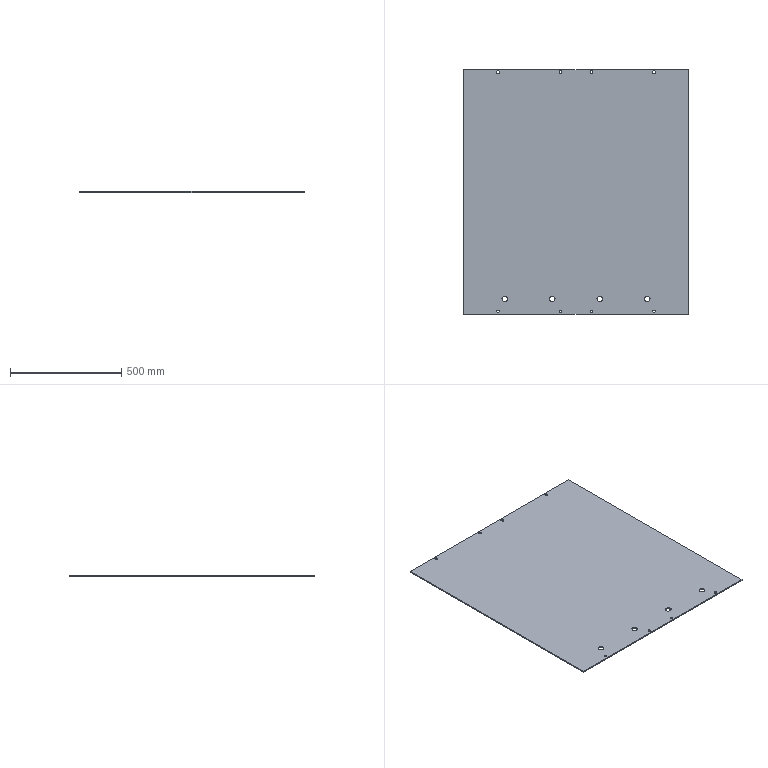Part | STEP file | 750038315 | 1 solid | 38 faces | box 1009 x 1100 x 5 mm | volume 5535001 mm3 | cylinder 24 | plane 14 | commonest cylinder face diameters 11 x16 25 x8
STEP:
#1=CARTESIAN_POINT('',(307.5,70.,0.));
#2=VERTEX_POINT('',#1);
#3=CARTESIAN_POINT('',(332.5,70.,0.));
#4=VERTEX_POINT('',#3);
#5=CARTESIAN_POINT('',(320.,70.,0.));
#6=DIRECTION('',(0.,0.,1.));
#7=DIRECTION('',(1.,0.,0.));
#8=AXIS2_PLACEMENT_3D('',#5,#6,#7);
#9=CIRCLE('',#8,12.5);
#10=EDGE_CURVE('',#2,#4,#9,.T.);
#11=ORIENTED_EDGE('',*,*,#10,.F.);
#12=CARTESIAN_POINT('',(307.5,70.,5.));
#13=VERTEX_POINT('',#12);
#14=CARTESIAN_POINT('',(307.5,70.,-1487.684));
#15=DIRECTION('',(0.,0.,1.));
#16=VECTOR('',#15,1000.);
#17=LINE('',#14,#16);
#18=EDGE_CURVE('',#2,#13,#17,.T.);
#19=ORIENTED_EDGE('',*,*,#18,.T.);
#20=CARTESIAN_POINT('',(332.5,70.,5.));
#21=VERTEX_POINT('',#20);
#22=CARTESIAN_POINT('',(320.,70.,5.));
#23=DIRECTION('',(0.,0.,-1.));
#24=DIRECTION('',(1.,0.,0.));
#25=AXIS2_PLACEMENT_3D('',#22,#23,#24);
#26=CIRCLE('',#25,12.5);
#27=EDGE_CURVE('',#21,#13,#26,.T.);
#28=ORIENTED_EDGE('',*,*,#27,.F.);
#29=CARTESIAN_POINT('',(332.5,70.,-1487.684));
#30=DIRECTION('',(0.,0.,1.));
#31=VECTOR('',#30,1000.);
#32=LINE('',#29,#31);
#33=EDGE_CURVE('',#4,#21,#32,.T.);
#34=ORIENTED_EDGE('',*,*,#33,.F.);
#35=EDGE_LOOP('',(#11,#19,#28,#34));
#36=FACE_OUTER_BOUND('',#35,.T.);
#37=CARTESIAN_POINT('',(320.,70.,-1487.684));
#38=DIRECTION('',(0.,0.,1.));
#39=DIRECTION('',(1.,0.,0.));
#40=AXIS2_PLACEMENT_3D('',#37,#38,#39);
#41=CYLINDRICAL_SURFACE('',#40,12.5);
#42=ADVANCED_FACE('',(#36),#41,.F.);
#43=CARTESIAN_POINT('',(94.167,70.,0.));
#44=VERTEX_POINT('',#43);
#45=CARTESIAN_POINT('',(119.167,70.,0.));
#46=VERTEX_POINT('',#45);
#47=CARTESIAN_POINT('',(106.667,70.,0.));
#48=DIRECTION('',(0.,0.,1.));
#49=DIRECTION('',(1.,0.,0.));
#50=AXIS2_PLACEMENT_3D('',#47,#48,#49);
#51=CIRCLE('',#50,12.5);
#52=EDGE_CURVE('',#44,#46,#51,.T.);
#53=ORIENTED_EDGE('',*,*,#52,.F.);
#54=CARTESIAN_POINT('',(94.167,70.,5.));
#55=VERTEX_POINT('',#54);
#56=CARTESIAN_POINT('',(94.167,70.,-1487.684));
#57=DIRECTION('',(0.,0.,1.));
#58=VECTOR('',#57,1000.);
#59=LINE('',#56,#58);
#60=EDGE_CURVE('',#44,#55,#59,.T.);
#61=ORIENTED_EDGE('',*,*,#60,.T.);
#62=CARTESIAN_POINT('',(119.167,70.,5.));
#63=VERTEX_POINT('',#62);
#64=CARTESIAN_POINT('',(106.667,70.,5.));
#65=DIRECTION('',(0.,0.,-1.));
#66=DIRECTION('',(1.,0.,0.));
#67=AXIS2_PLACEMENT_3D('',#64,#65,#66);
#68=CIRCLE('',#67,12.5);
#69=EDGE_CURVE('',#63,#55,#68,.T.);
#70=ORIENTED_EDGE('',*,*,#69,.F.);
#71=CARTESIAN_POINT('',(119.167,70.,-1487.684));
#72=DIRECTION('',(0.,0.,1.));
#73=VECTOR('',#72,1000.);
#74=LINE('',#71,#73);
#75=EDGE_CURVE('',#46,#63,#74,.T.);
#76=ORIENTED_EDGE('',*,*,#75,.F.);
#77=EDGE_LOOP('',(#53,#61,#70,#76));
#78=FACE_OUTER_BOUND('',#77,.T.);
#79=CARTESIAN_POINT('',(106.667,70.,-1487.684));
#80=DIRECTION('',(0.,0.,1.));
#81=DIRECTION('',(1.,0.,0.));
#82=AXIS2_PLACEMENT_3D('',#79,#80,#81);
#83=CYLINDRICAL_SURFACE('',#82,12.5);
#84=ADVANCED_FACE('',(#78),#83,.F.);
#85=CARTESIAN_POINT('',(-119.167,70.,0.));
#86=VERTEX_POINT('',#85);
#87=CARTESIAN_POINT('',(-94.167,70.,0.));
#88=VERTEX_POINT('',#87);
#89=CARTESIAN_POINT('',(-106.667,70.,0.));
#90=DIRECTION('',(0.,0.,1.));
#91=DIRECTION('',(1.,0.,0.));
#92=AXIS2_PLACEMENT_3D('',#89,#90,#91);
#93=CIRCLE('',#92,12.5);
#94=EDGE_CURVE('',#86,#88,#93,.T.);
#95=ORIENTED_EDGE('',*,*,#94,.F.);
#96=CARTESIAN_POINT('',(-119.167,70.,5.));
#97=VERTEX_POINT('',#96);
#98=CARTESIAN_POINT('',(-119.167,70.,-1487.684));
#99=DIRECTION('',(0.,0.,1.));
#100=VECTOR('',#99,1000.);
#101=LINE('',#98,#100);
#102=EDGE_CURVE('',#86,#97,#101,.T.);
#103=ORIENTED_EDGE('',*,*,#102,.T.);
#104=CARTESIAN_POINT('',(-94.167,70.,5.));
#105=VERTEX_POINT('',#104);
#106=CARTESIAN_POINT('',(-106.667,70.,5.));
#107=DIRECTION('',(0.,0.,-1.));
#108=DIRECTION('',(1.,0.,0.));
#109=AXIS2_PLACEMENT_3D('',#106,#107,#108);
#110=CIRCLE('',#109,12.5);
#111=EDGE_CURVE('',#105,#97,#110,.T.);
#112=ORIENTED_EDGE('',*,*,#111,.F.);
#113=CARTESIAN_POINT('',(-94.167,70.,-1487.684));
#114=DIRECTION('',(0.,0.,1.));
#115=VECTOR('',#114,1000.);
#116=LINE('',#113,#115);
#117=EDGE_CURVE('',#88,#105,#116,.T.);
#118=ORIENTED_EDGE('',*,*,#117,.F.);
#119=EDGE_LOOP('',(#95,#103,#112,#118));
#120=FACE_OUTER_BOUND('',#119,.T.);
#121=CARTESIAN_POINT('',(-106.667,70.,-1487.684));
#122=DIRECTION('',(0.,0.,1.));
#123=DIRECTION('',(1.,0.,0.));
#124=AXIS2_PLACEMENT_3D('',#121,#122,#123);
#125=CYLINDRICAL_SURFACE('',#124,12.5);
#126=ADVANCED_FACE('',(#120),#125,.F.);
#127=CARTESIAN_POINT('',(-332.5,70.,0.));
#128=VERTEX_POINT('',#127);
#129=CARTESIAN_POINT('',(-307.5,70.,0.));
#130=VERTEX_POINT('',#129);
#131=CARTESIAN_POINT('',(-320.,70.,0.));
#132=DIRECTION('',(0.,0.,1.));
#133=DIRECTION('',(1.,0.,0.));
#134=AXIS2_PLACEMENT_3D('',#131,#132,#133);
#135=CIRCLE('',#134,12.5);
#136=EDGE_CURVE('',#128,#130,#135,.T.);
#137=ORIENTED_EDGE('',*,*,#136,.F.);
#138=CARTESIAN_POINT('',(-332.5,70.,5.));
#139=VERTEX_POINT('',#138);
#140=CARTESIAN_POINT('',(-332.5,70.,-1487.684));
#141=DIRECTION('',(0.,0.,1.));
#142=VECTOR('',#141,1000.);
#143=LINE('',#140,#142);
#144=EDGE_CURVE('',#128,#139,#143,.T.);
#145=ORIENTED_EDGE('',*,*,#144,.T.);
#146=CARTESIAN_POINT('',(-307.5,70.,5.));
#147=VERTEX_POINT('',#146);
#148=CARTESIAN_POINT('',(-320.,70.,5.));
#149=DIRECTION('',(0.,0.,-1.));
#150=DIRECTION('',(1.,0.,0.));
#151=AXIS2_PLACEMENT_3D('',#148,#149,#150);
#152=CIRCLE('',#151,12.5);
#153=EDGE_CURVE('',#147,#139,#152,.T.);
#154=ORIENTED_EDGE('',*,*,#153,.F.);
#155=CARTESIAN_POINT('',(-307.5,70.,-1487.684));
#156=DIRECTION('',(0.,0.,1.));
#157=VECTOR('',#156,1000.);
#158=LINE('',#155,#157);
#159=EDGE_CURVE('',#130,#147,#158,.T.);
#160=ORIENTED_EDGE('',*,*,#159,.F.);
#161=EDGE_LOOP('',(#137,#145,#154,#160));
#162=FACE_OUTER_BOUND('',#161,.T.);
#163=CARTESIAN_POINT('',(-320.,70.,-1487.684));
#164=DIRECTION('',(0.,0.,1.));
#165=DIRECTION('',(1.,0.,0.));
#166=AXIS2_PLACEMENT_3D('',#163,#164,#165);
#167=CYLINDRICAL_SURFACE('',#166,12.5);
#168=ADVANCED_FACE('',(#162),#167,.F.);
#169=CARTESIAN_POINT('',(75.5,14.,5.));
#170=VERTEX_POINT('',#169);
#171=CARTESIAN_POINT('',(64.5,14.,5.));
#172=VERTEX_POINT('',#171);
#173=CARTESIAN_POINT('',(70.,14.,5.));
#174=DIRECTION('',(0.,0.,-1.));
#175=DIRECTION('',(-1.,0.,0.));
#176=AXIS2_PLACEMENT_3D('',#173,#174,#175);
#177=CIRCLE('',#176,5.5);
#178=EDGE_CURVE('',#170,#172,#177,.T.);
#179=ORIENTED_EDGE('',*,*,#178,.F.);
#180=CARTESIAN_POINT('',(75.5,14.,0.));
#181=VERTEX_POINT('',#180);
#182=CARTESIAN_POINT('',(75.5,14.,1492.684));
#183=DIRECTION('',(0.,0.,-1.));
#184=VECTOR('',#183,1000.);
#185=LINE('',#182,#184);
#186=EDGE_CURVE('',#170,#181,#185,.T.);
#187=ORIENTED_EDGE('',*,*,#186,.T.);
#188=CARTESIAN_POINT('',(64.5,14.,0.));
#189=VERTEX_POINT('',#188);
#190=CARTESIAN_POINT('',(70.,14.,0.));
#191=DIRECTION('',(0.,0.,1.));
#192=DIRECTION('',(-1.,0.,0.));
#193=AXIS2_PLACEMENT_3D('',#190,#191,#192);
#194=CIRCLE('',#193,5.5);
#195=EDGE_CURVE('',#189,#181,#194,.T.);
#196=ORIENTED_EDGE('',*,*,#195,.F.);
#197=CARTESIAN_POINT('',(64.5,14.,1492.684));
#198=DIRECTION('',(0.,0.,-1.));
#199=VECTOR('',#198,1000.);
#200=LINE('',#197,#199);
#201=EDGE_CURVE('',#172,#189,#200,.T.);
#202=ORIENTED_EDGE('',*,*,#201,.F.);
#203=EDGE_LOOP('',(#179,#187,#196,#202));
#204=FACE_OUTER_BOUND('',#203,.T.);
#205=CARTESIAN_POINT('',(70.,14.,1492.684));
#206=DIRECTION('',(0.,0.,-1.));
#207=DIRECTION('',(-1.,0.,0.));
#208=AXIS2_PLACEMENT_3D('',#205,#206,#207);
#209=CYLINDRICAL_SURFACE('',#208,5.5);
#210=ADVANCED_FACE('',(#204),#209,.F.);
#211=CARTESIAN_POINT('',(-64.5,14.,5.));
#212=VERTEX_POINT('',#211);
#213=CARTESIAN_POINT('',(-75.5,14.,5.));
#214=VERTEX_POINT('',#213);
#215=CARTESIAN_POINT('',(-70.,14.,5.));
#216=DIRECTION('',(0.,0.,-1.));
#217=DIRECTION('',(-1.,0.,0.));
#218=AXIS2_PLACEMENT_3D('',#215,#216,#217);
#219=CIRCLE('',#218,5.5);
#220=EDGE_CURVE('',#212,#214,#219,.T.);
#221=ORIENTED_EDGE('',*,*,#220,.F.);
#222=CARTESIAN_POINT('',(-64.5,14.,0.));
#223=VERTEX_POINT('',#222);
#224=CARTESIAN_POINT('',(-64.5,14.,1492.684));
#225=DIRECTION('',(0.,0.,-1.));
#226=VECTOR('',#225,1000.);
#227=LINE('',#224,#226);
#228=EDGE_CURVE('',#212,#223,#227,.T.);
#229=ORIENTED_EDGE('',*,*,#228,.T.);
#230=CARTESIAN_POINT('',(-75.5,14.,0.));
#231=VERTEX_POINT('',#230);
#232=CARTESIAN_POINT('',(-70.,14.,0.));
#233=DIRECTION('',(0.,0.,1.));
#234=DIRECTION('',(-1.,0.,0.));
#235=AXIS2_PLACEMENT_3D('',#232,#233,#234);
#236=CIRCLE('',#235,5.5);
#237=EDGE_CURVE('',#231,#223,#236,.T.);
#238=ORIENTED_EDGE('',*,*,#237,.F.);
#239=CARTESIAN_POINT('',(-75.5,14.,1492.684));
#240=DIRECTION('',(0.,0.,-1.));
#241=VECTOR('',#240,1000.);
#242=LINE('',#239,#241);
#243=EDGE_CURVE('',#214,#231,#242,.T.);
#244=ORIENTED_EDGE('',*,*,#243,.F.);
#245=EDGE_LOOP('',(#221,#229,#238,#244));
#246=FACE_OUTER_BOUND('',#245,.T.);
#247=CARTESIAN_POINT('',(-70.,14.,1492.684));
#248=DIRECTION('',(0.,0.,-1.));
#249=DIRECTION('',(-1.,0.,0.));
#250=AXIS2_PLACEMENT_3D('',#247,#248,#249);
#251=CYLINDRICAL_SURFACE('',#250,5.5);
#252=ADVANCED_FACE('',(#246),#251,.F.);
#253=CARTESIAN_POINT('',(-344.5,14.,5.));
#254=VERTEX_POINT('',#253);
#255=CARTESIAN_POINT('',(-355.5,14.,5.));
#256=VERTEX_POINT('',#255);
#257=CARTESIAN_POINT('',(-350.,14.,5.));
#258=DIRECTION('',(0.,0.,-1.));
#259=DIRECTION('',(-1.,0.,0.));
#260=AXIS2_PLACEMENT_3D('',#257,#258,#259);
#261=CIRCLE('',#260,5.5);
#262=EDGE_CURVE('',#254,#256,#261,.T.);
#263=ORIENTED_EDGE('',*,*,#262,.F.);
#264=CARTESIAN_POINT('',(-344.5,14.,0.));
#265=VERTEX_POINT('',#264);
#266=CARTESIAN_POINT('',(-344.5,14.,1492.684));
#267=DIRECTION('',(0.,0.,-1.));
#268=VECTOR('',#267,1000.);
#269=LINE('',#266,#268);
#270=EDGE_CURVE('',#254,#265,#269,.T.);
#271=ORIENTED_EDGE('',*,*,#270,.T.);
#272=CARTESIAN_POINT('',(-355.5,14.,0.));
#273=VERTEX_POINT('',#272);
#274=CARTESIAN_POINT('',(-350.,14.,0.));
#275=DIRECTION('',(0.,0.,1.));
#276=DIRECTION('',(-1.,0.,0.));
#277=AXIS2_PLACEMENT_3D('',#274,#275,#276);
#278=CIRCLE('',#277,5.5);
#279=EDGE_CURVE('',#273,#265,#278,.T.);
#280=ORIENTED_EDGE('',*,*,#279,.F.);
#281=CARTESIAN_POINT('',(-355.5,14.,1492.684));
#282=DIRECTION('',(0.,0.,-1.));
#283=VECTOR('',#282,1000.);
#284=LINE('',#281,#283);
#285=EDGE_CURVE('',#256,#273,#284,.T.);
#286=ORIENTED_EDGE('',*,*,#285,.F.);
#287=EDGE_LOOP('',(#263,#271,#280,#286));
#288=FACE_OUTER_BOUND('',#287,.T.);
#289=CARTESIAN_POINT('',(-350.,14.,1492.684));
#290=DIRECTION('',(0.,0.,-1.));
#291=DIRECTION('',(-1.,0.,0.));
#292=AXIS2_PLACEMENT_3D('',#289,#290,#291);
#293=CYLINDRICAL_SURFACE('',#292,5.5);
#294=ADVANCED_FACE('',(#288),#293,.F.);
#295=CARTESIAN_POINT('',(355.5,14.,5.));
#296=VERTEX_POINT('',#295);
#297=CARTESIAN_POINT('',(344.5,14.,5.));
#298=VERTEX_POINT('',#297);
#299=CARTESIAN_POINT('',(350.,14.,5.));
#300=DIRECTION('',(0.,0.,-1.));
#301=DIRECTION('',(-1.,0.,0.));
#302=AXIS2_PLACEMENT_3D('',#299,#300,#301);
#303=CIRCLE('',#302,5.5);
#304=EDGE_CURVE('',#296,#298,#303,.T.);
#305=ORIENTED_EDGE('',*,*,#304,.F.);
#306=CARTESIAN_POINT('',(355.5,14.,0.));
#307=VERTEX_POINT('',#306);
#308=CARTESIAN_POINT('',(355.5,14.,1492.684));
#309=DIRECTION('',(0.,0.,-1.));
#310=VECTOR('',#309,1000.);
#311=LINE('',#308,#310);
#312=EDGE_CURVE('',#296,#307,#311,.T.);
#313=ORIENTED_EDGE('',*,*,#312,.T.);
#314=CARTESIAN_POINT('',(344.5,14.,0.));
#315=VERTEX_POINT('',#314);
#316=CARTESIAN_POINT('',(350.,14.,0.));
#317=DIRECTION('',(0.,0.,1.));
#318=DIRECTION('',(-1.,0.,0.));
#319=AXIS2_PLACEMENT_3D('',#316,#317,#318);
#320=CIRCLE('',#319,5.5);
#321=EDGE_CURVE('',#315,#307,#320,.T.);
#322=ORIENTED_EDGE('',*,*,#321,.F.);
#323=CARTESIAN_POINT('',(344.5,14.,1492.684));
#324=DIRECTION('',(0.,0.,-1.));
#325=VECTOR('',#324,1000.);
#326=LINE('',#323,#325);
#327=EDGE_CURVE('',#298,#315,#326,.T.);
#328=ORIENTED_EDGE('',*,*,#327,.F.);
#329=EDGE_LOOP('',(#305,#313,#322,#328));
#330=FACE_OUTER_BOUND('',#329,.T.);
#331=CARTESIAN_POINT('',(350.,14.,1492.684));
#332=DIRECTION('',(0.,0.,-1.));
#333=DIRECTION('',(-1.,0.,0.));
#334=AXIS2_PLACEMENT_3D('',#331,#332,#333);
#335=CYLINDRICAL_SURFACE('',#334,5.5);
#336=ADVANCED_FACE('',(#330),#335,.F.);
#337=CARTESIAN_POINT('',(-355.5,1090.,0.));
#338=VERTEX_POINT('',#337);
#339=CARTESIAN_POINT('',(-355.5,1086.,0.));
#340=VERTEX_POINT('',#339);
#341=CARTESIAN_POINT('',(-355.5,0.,0.));
#342=DIRECTION('',(0.,-1.,0.));
#343=VECTOR('',#342,1000.);
#344=LINE('',#341,#343);
#345=EDGE_CURVE('',#338,#340,#344,.T.);
#346=ORIENTED_EDGE('',*,*,#345,.T.);
#347=CARTESIAN_POINT('',(-344.5,1086.,0.));
#348=VERTEX_POINT('',#347);
#349=CARTESIAN_POINT('',(-350.,1086.,0.));
#350=DIRECTION('',(0.,0.,1.));
#351=DIRECTION('',(-1.,0.,0.));
#352=AXIS2_PLACEMENT_3D('',#349,#350,#351);
#353=CIRCLE('',#352,5.5);
#354=EDGE_CURVE('',#340,#348,#353,.T.);
#355=ORIENTED_EDGE('',*,*,#354,.T.);
#356=CARTESIAN_POINT('',(-344.5,1090.,0.));
#357=VERTEX_POINT('',#356);
#358=CARTESIAN_POINT('',(-344.5,0.,0.));
#359=DIRECTION('',(0.,1.,0.));
#360=VECTOR('',#359,1000.);
#361=LINE('',#358,#360);
#362=EDGE_CURVE('',#348,#357,#361,.T.);
#363=ORIENTED_EDGE('',*,*,#362,.T.);
#364=CARTESIAN_POINT('',(-350.,1090.,0.));
#365=DIRECTION('',(0.,0.,1.));
#366=DIRECTION('',(-1.,0.,0.));
#367=AXIS2_PLACEMENT_3D('',#364,#365,#366);
#368=CIRCLE('',#367,5.5);
#369=EDGE_CURVE('',#357,#338,#368,.T.);
#370=ORIENTED_EDGE('',*,*,#369,.T.);
#371=EDGE_LOOP('',(#346,#355,#363,#370));
#372=FACE_BOUND('',#371,.T.);
#373=CARTESIAN_POINT('',(-75.5,1090.,0.));
#374=VERTEX_POINT('',#373);
#375=CARTESIAN_POINT('',(-75.5,1086.,0.));
#376=VERTEX_POINT('',#375);
#377=CARTESIAN_POINT('',(-75.5,0.,0.));
#378=DIRECTION('',(0.,-1.,0.));
#379=VECTOR('',#378,1000.);
#380=LINE('',#377,#379);
#381=EDGE_CURVE('',#374,#376,#380,.T.);
#382=ORIENTED_EDGE('',*,*,#381,.T.);
#383=CARTESIAN_POINT('',(-64.5,1086.,0.));
#384=VERTEX_POINT('',#383);
#385=CARTESIAN_POINT('',(-70.,1086.,0.));
#386=DIRECTION('',(0.,0.,1.));
#387=DIRECTION('',(-1.,0.,0.));
#388=AXIS2_PLACEMENT_3D('',#385,#386,#387);
#389=CIRCLE('',#388,5.5);
#390=EDGE_CURVE('',#376,#384,#389,.T.);
#391=ORIENTED_EDGE('',*,*,#390,.T.);
#392=CARTESIAN_POINT('',(-64.5,1090.,0.));
#393=VERTEX_POINT('',#392);
#394=CARTESIAN_POINT('',(-64.5,0.,0.));
#395=DIRECTION('',(0.,1.,0.));
#396=VECTOR('',#395,1000.);
#397=LINE('',#394,#396);
#398=EDGE_CURVE('',#384,#393,#397,.T.);
#399=ORIENTED_EDGE('',*,*,#398,.T.);
#400=CARTESIAN_POINT('',(-70.,1090.,0.));
#401=DIRECTION('',(0.,0.,1.));
#402=DIRECTION('',(-1.,0.,0.));
#403=AXIS2_PLACEMENT_3D('',#400,#401,#402);
#404=CIRCLE('',#403,5.5);
#405=EDGE_CURVE('',#393,#374,#404,.T.);
#406=ORIENTED_EDGE('',*,*,#405,.T.);
#407=EDGE_LOOP('',(#382,#391,#399,#406));
#408=FACE_BOUND('',#407,.T.);
#409=CARTESIAN_POINT('',(64.5,1090.,0.));
#410=VERTEX_POINT('',#409);
#411=CARTESIAN_POINT('',(64.5,1086.,0.));
#412=VERTEX_POINT('',#411);
#413=CARTESIAN_POINT('',(64.5,0.,0.));
#414=DIRECTION('',(0.,-1.,0.));
#415=VECTOR('',#414,1000.);
#416=LINE('',#413,#415);
#417=EDGE_CURVE('',#410,#412,#416,.T.);
#418=ORIENTED_EDGE('',*,*,#417,.T.);
#419=CARTESIAN_POINT('',(75.5,1086.,0.));
#420=VERTEX_POINT('',#419);
#421=CARTESIAN_POINT('',(70.,1086.,0.));
#422=DIRECTION('',(0.,0.,1.));
#423=DIRECTION('',(-1.,0.,0.));
#424=AXIS2_PLACEMENT_3D('',#421,#422,#423);
#425=CIRCLE('',#424,5.5);
#426=EDGE_CURVE('',#412,#420,#425,.T.);
#427=ORIENTED_EDGE('',*,*,#426,.T.);
#428=CARTESIAN_POINT('',(75.5,1090.,0.));
#429=VERTEX_POINT('',#428);
#430=CARTESIAN_POINT('',(75.5,0.,0.));
#431=DIRECTION('',(0.,1.,0.));
#432=VECTOR('',#431,1000.);
#433=LINE('',#430,#432);
#434=EDGE_CURVE('',#420,#429,#433,.T.);
#435=ORIENTED_EDGE('',*,*,#434,.T.);
#436=CARTESIAN_POINT('',(70.,1090.,0.));
#437=DIRECTION('',(0.,0.,1.));
#438=DIRECTION('',(-1.,0.,0.));
#439=AXIS2_PLACEMENT_3D('',#436,#437,#438);
#440=CIRCLE('',#439,5.5);
#441=EDGE_CURVE('',#429,#410,#440,.T.);
#442=ORIENTED_EDGE('',*,*,#441,.T.);
#443=EDGE_LOOP('',(#418,#427,#435,#442));
#444=FACE_BOUND('',#443,.T.);
#445=CARTESIAN_POINT('',(344.5,1090.,0.));
#446=VERTEX_POINT('',#445);
#447=CARTESIAN_POINT('',(344.5,1086.,0.));
#448=VERTEX_POINT('',#447);
#449=CARTESIAN_POINT('',(344.5,0.,0.));
#450=DIRECTION('',(0.,-1.,0.));
#451=VECTOR('',#450,1000.);
#452=LINE('',#449,#451);
#453=EDGE_CURVE('',#446,#448,#452,.T.);
#454=ORIENTED_EDGE('',*,*,#453,.T.);
#455=CARTESIAN_POINT('',(355.5,1086.,0.));
#456=VERTEX_POINT('',#455);
#457=CARTESIAN_POINT('',(350.,1086.,0.));
#458=DIRECTION('',(0.,0.,1.));
#459=DIRECTION('',(-1.,0.,0.));
#460=AXIS2_PLACEMENT_3D('',#457,#458,#459);
#461=CIRCLE('',#460,5.5);
#462=EDGE_CURVE('',#448,#456,#461,.T.);
#463=ORIENTED_EDGE('',*,*,#462,.T.);
#464=CARTESIAN_POINT('',(355.5,1090.,0.));
#465=VERTEX_POINT('',#464);
#466=CARTESIAN_POINT('',(355.5,0.,0.));
#467=DIRECTION('',(0.,1.,0.));
#468=VECTOR('',#467,1000.);
#469=LINE('',#466,#468);
#470=EDGE_CURVE('',#456,#465,#469,.T.);
#471=ORIENTED_EDGE('',*,*,#470,.T.);
#472=CARTESIAN_POINT('',(350.,1090.,0.));
#473=DIRECTION('',(0.,0.,1.));
#474=DIRECTION('',(-1.,0.,0.));
#475=AXIS2_PLACEMENT_3D('',#472,#473,#474);
#476=CIRCLE('',#475,5.5);
#477=EDGE_CURVE('',#465,#446,#476,.T.);
#478=ORIENTED_EDGE('',*,*,#477,.T.);
#479=EDGE_LOOP('',(#454,#463,#471,#478));
#480=FACE_BOUND('',#479,.T.);
#481=CARTESIAN_POINT('',(-504.5,1100.,0.));
#482=VERTEX_POINT('',#481);
#483=CARTESIAN_POINT('',(504.5,1100.,0.));
#484=VERTEX_POINT('',#483);
#485=CARTESIAN_POINT('',(0.,1100.,0.));
#486=DIRECTION('',(1.,0.,0.));
#487=VECTOR('',#486,1000.);
#488=LINE('',#485,#487);
#489=EDGE_CURVE('',#482,#484,#488,.T.);
#490=ORIENTED_EDGE('',*,*,#489,.T.);
#491=CARTESIAN_POINT('',(504.5,0.,0.));
#492=VERTEX_POINT('',#491);
#493=CARTESIAN_POINT('',(504.5,0.,0.));
#494=DIRECTION('',(0.,-1.,0.));
#495=VECTOR('',#494,1000.);
#496=LINE('',#493,#495);
#497=EDGE_CURVE('',#484,#492,#496,.T.);
#498=ORIENTED_EDGE('',*,*,#497,.T.);
#499=CARTESIAN_POINT('',(-504.5,0.,0.));
#500=VERTEX_POINT('',#499);
#501=CARTESIAN_POINT('',(0.,0.,0.));
#502=DIRECTION('',(-1.,0.,0.));
#503=VECTOR('',#502,1000.);
#504=LINE('',#501,#503);
#505=EDGE_CURVE('',#492,#500,#504,.T.);
#506=ORIENTED_EDGE('',*,*,#505,.T.);
#507=CARTESIAN_POINT('',(-504.5,0.,0.));
#508=DIRECTION('',(0.,1.,0.));
#509=VECTOR('',#508,1000.);
#510=LINE('',#507,#509);
#511=EDGE_CURVE('',#500,#482,#510,.T.);
#512=ORIENTED_EDGE('',*,*,#511,.T.);
#513=EDGE_LOOP('',(#490,#498,#506,#512));
#514=FACE_OUTER_BOUND('',#513,.T.);
#515=CARTESIAN_POINT('',(320.,70.,0.));
#516=DIRECTION('',(0.,0.,1.));
#517=DIRECTION('',(1.,0.,0.));
#518=AXIS2_PLACEMENT_3D('',#515,#516,#517);
#519=CIRCLE('',#518,12.5);
#520=EDGE_CURVE('',#4,#2,#519,.T.);
#521=ORIENTED_EDGE('',*,*,#520,.T.);
#522=ORIENTED_EDGE('',*,*,#10,.T.);
#523=EDGE_LOOP('',(#521,#522));
#524=FACE_BOUND('',#523,.T.);
#525=CARTESIAN_POINT('',(106.667,70.,0.));
#526=DIRECTION('',(0.,0.,1.));
#527=DIRECTION('',(1.,0.,0.));
#528=AXIS2_PLACEMENT_3D('',#525,#526,#527);
#529=CIRCLE('',#528,12.5);
#530=EDGE_CURVE('',#46,#44,#529,.T.);
#531=ORIENTED_EDGE('',*,*,#530,.T.);
#532=ORIENTED_EDGE('',*,*,#52,.T.);
#533=EDGE_LOOP('',(#531,#532));
#534=FACE_BOUND('',#533,.T.);
#535=CARTESIAN_POINT('',(-106.667,70.,0.));
#536=DIRECTION('',(0.,0.,1.));
#537=DIRECTION('',(1.,0.,0.));
#538=AXIS2_PLACEMENT_3D('',#535,#536,#537);
#539=CIRCLE('',#538,12.5);
#540=EDGE_CURVE('',#88,#86,#539,.T.);
#541=ORIENTED_EDGE('',*,*,#540,.T.);
#542=ORIENTED_EDGE('',*,*,#94,.T.);
#543=EDGE_LOOP('',(#541,#542));
#544=FACE_BOUND('',#543,.T.);
#545=CARTESIAN_POINT('',(-320.,70.,0.));
#546=DIRECTION('',(0.,0.,1.));
#547=DIRECTION('',(1.,0.,0.));
#548=AXIS2_PLACEMENT_3D('',#545,#546,#547);
#549=CIRCLE('',#548,12.5);
#550=EDGE_CURVE('',#130,#128,#549,.T.);
#551=ORIENTED_EDGE('',*,*,#550,.T.);
#552=ORIENTED_EDGE('',*,*,#136,.T.);
#553=EDGE_LOOP('',(#551,#552));
#554=FACE_BOUND('',#553,.T.);
#555=ORIENTED_EDGE('',*,*,#195,.T.);
#556=CARTESIAN_POINT('',(70.,14.,0.));
#557=DIRECTION('',(0.,0.,1.));
#558=DIRECTION('',(-1.,0.,0.));
#559=AXIS2_PLACEMENT_3D('',#556,#557,#558);
#560=CIRCLE('',#559,5.5);
#561=EDGE_CURVE('',#181,#189,#560,.T.);
#562=ORIENTED_EDGE('',*,*,#561,.T.);
#563=EDGE_LOOP('',(#555,#562));
#564=FACE_BOUND('',#563,.T.);
#565=ORIENTED_EDGE('',*,*,#237,.T.);
#566=CARTESIAN_POINT('',(-70.,14.,0.));
#567=DIRECTION('',(0.,0.,1.));
#568=DIRECTION('',(-1.,0.,0.));
#569=AXIS2_PLACEMENT_3D('',#566,#567,#568);
#570=CIRCLE('',#569,5.5);
#571=EDGE_CURVE('',#223,#231,#570,.T.);
#572=ORIENTED_EDGE('',*,*,#571,.T.);
#573=EDGE_LOOP('',(#565,#572));
#574=FACE_BOUND('',#573,.T.);
#575=ORIENTED_EDGE('',*,*,#279,.T.);
#576=CARTESIAN_POINT('',(-350.,14.,0.));
#577=DIRECTION('',(0.,0.,1.));
#578=DIRECTION('',(-1.,0.,0.));
#579=AXIS2_PLACEMENT_3D('',#576,#577,#578);
#580=CIRCLE('',#579,5.5);
#581=EDGE_CURVE('',#265,#273,#580,.T.);
#582=ORIENTED_EDGE('',*,*,#581,.T.);
#583=EDGE_LOOP('',(#575,#582));
#584=FACE_BOUND('',#583,.T.);
#585=ORIENTED_EDGE('',*,*,#321,.T.);
#586=CARTESIAN_POINT('',(350.,14.,0.));
#587=DIRECTION('',(0.,0.,1.));
#588=DIRECTION('',(-1.,0.,0.));
#589=AXIS2_PLACEMENT_3D('',#586,#587,#588);
#590=CIRCLE('',#589,5.5);
#591=EDGE_CURVE('',#307,#315,#590,.T.);
#592=ORIENTED_EDGE('',*,*,#591,.T.);
#593=EDGE_LOOP('',(#585,#592));
#594=FACE_BOUND('',#593,.T.);
#595=CARTESIAN_POINT('',(0.,0.,0.));
#596=DIRECTION('',(0.,0.,-1.));
#597=DIRECTION('',(-1.,0.,0.));
#598=AXIS2_PLACEMENT_3D('',#595,#596,#597);
#599=PLANE('',#598);
#600=ADVANCED_FACE('',(#372,#408,#444,#480,#514,#524,#534,#544,#554,#564,#574,#584,#594),#599,.T.);
#601=CARTESIAN_POINT('',(-344.5,1086.,5.));
#602=VERTEX_POINT('',#601);
#603=CARTESIAN_POINT('',(-344.5,1086.,1492.684));
#604=DIRECTION('',(0.,0.,1.));
#605=VECTOR('',#604,1000.);
#606=LINE('',#603,#605);
#607=EDGE_CURVE('',#348,#602,#606,.T.);
#608=ORIENTED_EDGE('',*,*,#607,.F.);
#609=ORIENTED_EDGE('',*,*,#354,.F.);
#610=CARTESIAN_POINT('',(-355.5,1086.,5.));
#611=VERTEX_POINT('',#610);
#612=CARTESIAN_POINT('',(-355.5,1086.,1492.684));
#613=DIRECTION('',(0.,0.,-1.));
#614=VECTOR('',#613,1000.);
#615=LINE('',#612,#614);
#616=EDGE_CURVE('',#611,#340,#615,.T.);
#617=ORIENTED_EDGE('',*,*,#616,.F.);
#618=CARTESIAN_POINT('',(-350.,1086.,5.));
#619=DIRECTION('',(0.,0.,-1.));
#620=DIRECTION('',(-1.,0.,0.));
#621=AXIS2_PLACEMENT_3D('',#618,#619,#620);
#622=CIRCLE('',#621,5.5);
#623=EDGE_CURVE('',#602,#611,#622,.T.);
#624=ORIENTED_EDGE('',*,*,#623,.F.);
#625=EDGE_LOOP('',(#608,#609,#617,#624));
#626=FACE_OUTER_BOUND('',#625,.T.);
#627=CARTESIAN_POINT('',(-350.,1086.,1492.684));
#628=DIRECTION('',(0.,0.,-1.));
#629=DIRECTION('',(-1.,0.,0.));
#630=AXIS2_PLACEMENT_3D('',#627,#628,#629);
#631=CYLINDRICAL_SURFACE('',#630,5.5);
#632=ADVANCED_FACE('',(#626),#631,.F.);
#633=ORIENTED_EDGE('',*,*,#345,.F.);
#634=CARTESIAN_POINT('',(-355.5,1090.,5.));
#635=VERTEX_POINT('',#634);
#636=CARTESIAN_POINT('',(-355.5,1090.,1492.684));
#637=DIRECTION('',(0.,0.,1.));
#638=VECTOR('',#637,1000.);
#639=LINE('',#636,#638);
#640=EDGE_CURVE('',#338,#635,#639,.T.);
#641=ORIENTED_EDGE('',*,*,#640,.T.);
#642=CARTESIAN_POINT('',(-355.5,1090.,5.));
#643=DIRECTION('',(0.,-1.,0.));
#644=VECTOR('',#643,1000.);
#645=LINE('',#642,#644);
#646=EDGE_CURVE('',#635,#611,#645,.T.);
#647=ORIENTED_EDGE('',*,*,#646,.T.);
#648=ORIENTED_EDGE('',*,*,#616,.T.);
#649=EDGE_LOOP('',(#633,#641,#647,#648));
#650=FACE_OUTER_BOUND('',#649,.T.);
#651=CARTESIAN_POINT('',(-355.5,1090.,1492.684));
#652=DIRECTION('',(1.,0.,0.));
#653=DIRECTION('',(0.,0.,-1.));
#654=AXIS2_PLACEMENT_3D('',#651,#652,#653);
#655=PLANE('',#654);
#656=ADVANCED_FACE('',(#650),#655,.T.);
#657=ORIENTED_EDGE('',*,*,#640,.F.);
#658=ORIENTED_EDGE('',*,*,#369,.F.);
#659=CARTESIAN_POINT('',(-344.5,1090.,5.));
#660=VERTEX_POINT('',#659);
#661=CARTESIAN_POINT('',(-344.5,1090.,1492.684));
#662=DIRECTION('',(0.,0.,-1.));
#663=VECTOR('',#662,1000.);
#664=LINE('',#661,#663);
#665=EDGE_CURVE('',#660,#357,#664,.T.);
#666=ORIENTED_EDGE('',*,*,#665,.F.);
#667=CARTESIAN_POINT('',(-350.,1090.,5.));
#668=DIRECTION('',(0.,0.,-1.));
#669=DIRECTION('',(-1.,0.,0.));
#670=AXIS2_PLACEMENT_3D('',#667,#668,#669);
#671=CIRCLE('',#670,5.5);
#672=EDGE_CURVE('',#635,#660,#671,.T.);
#673=ORIENTED_EDGE('',*,*,#672,.F.);
#674=EDGE_LOOP('',(#657,#658,#666,#673));
#675=FACE_OUTER_BOUND('',#674,.T.);
#676=CARTESIAN_POINT('',(-350.,1090.,1492.684));
#677=DIRECTION('',(0.,0.,-1.));
#678=DIRECTION('',(-1.,0.,0.));
#679=AXIS2_PLACEMENT_3D('',#676,#677,#678);
#680=CYLINDRICAL_SURFACE('',#679,5.5);
#681=ADVANCED_FACE('',(#675),#680,.F.);
#682=ORIENTED_EDGE('',*,*,#362,.F.);
#683=ORIENTED_EDGE('',*,*,#607,.T.);
#684=CARTESIAN_POINT('',(-344.5,1086.,5.));
#685=DIRECTION('',(0.,1.,0.));
#686=VECTOR('',#685,1000.);
#687=LINE('',#684,#686);
#688=EDGE_CURVE('',#602,#660,#687,.T.);
#689=ORIENTED_EDGE('',*,*,#688,.T.);
#690=ORIENTED_EDGE('',*,*,#665,.T.);
#691=EDGE_LOOP('',(#682,#683,#689,#690));
#692=FACE_OUTER_BOUND('',#691,.T.);
#693=CARTESIAN_POINT('',(-344.5,1086.,1492.684));
#694=DIRECTION('',(-1.,0.,0.));
#695=DIRECTION('',(0.,0.,1.));
#696=AXIS2_PLACEMENT_3D('',#693,#694,#695);
#697=PLANE('',#696);
#698=ADVANCED_FACE('',(#692),#697,.T.);
#699=CARTESIAN_POINT('',(-64.5,1086.,5.));
#700=VERTEX_POINT('',#699);
#701=CARTESIAN_POINT('',(-64.5,1086.,1492.684));
#702=DIRECTION('',(0.,0.,1.));
#703=VECTOR('',#702,1000.);
#704=LINE('',#701,#703);
#705=EDGE_CURVE('',#384,#700,#704,.T.);
#706=ORIENTED_EDGE('',*,*,#705,.F.);
#707=ORIENTED_EDGE('',*,*,#390,.F.);
#708=CARTESIAN_POINT('',(-75.5,1086.,5.));
#709=VERTEX_POINT('',#708);
#710=CARTESIAN_POINT('',(-75.5,1086.,1492.684));
#711=DIRECTION('',(0.,0.,-1.));
#712=VECTOR('',#711,1000.);
#713=LINE('',#710,#712);
#714=EDGE_CURVE('',#709,#376,#713,.T.);
#715=ORIENTED_EDGE('',*,*,#714,.F.);
#716=CARTESIAN_POINT('',(-70.,1086.,5.));
#717=DIRECTION('',(0.,0.,-1.));
#718=DIRECTION('',(-1.,0.,0.));
#719=AXIS2_PLACEMENT_3D('',#716,#717,#718);
#720=CIRCLE('',#719,5.5);
#721=EDGE_CURVE('',#700,#709,#720,.T.);
#722=ORIENTED_EDGE('',*,*,#721,.F.);
#723=EDGE_LOOP('',(#706,#707,#715,#722));
#724=FACE_OUTER_BOUND('',#723,.T.);
#725=CARTESIAN_POINT('',(-70.,1086.,1492.684));
#726=DIRECTION('',(0.,0.,-1.));
#727=DIRECTION('',(-1.,0.,0.));
#728=AXIS2_PLACEMENT_3D('',#725,#726,#727);
#729=CYLINDRICAL_SURFACE('',#728,5.5);
#730=ADVANCED_FACE('',(#724),#729,.F.);
#731=ORIENTED_EDGE('',*,*,#381,.F.);
#732=CARTESIAN_POINT('',(-75.5,1090.,5.));
#733=VERTEX_POINT('',#732);
#734=CARTESIAN_POINT('',(-75.5,1090.,1492.684));
#735=DIRECTION('',(0.,0.,1.));
#736=VECTOR('',#735,1000.);
#737=LINE('',#734,#736);
#738=EDGE_CURVE('',#374,#733,#737,.T.);
#739=ORIENTED_EDGE('',*,*,#738,.T.);
#740=CARTESIAN_POINT('',(-75.5,1090.,5.));
#741=DIRECTION('',(0.,-1.,0.));
#742=VECTOR('',#741,1000.);
#743=LINE('',#740,#742);
#744=EDGE_CURVE('',#733,#709,#743,.T.);
#745=ORIENTED_EDGE('',*,*,#744,.T.);
#746=ORIENTED_EDGE('',*,*,#714,.T.);
#747=EDGE_LOOP('',(#731,#739,#745,#746));
#748=FACE_OUTER_BOUND('',#747,.T.);
#749=CARTESIAN_POINT('',(-75.5,1090.,1492.684));
#750=DIRECTION('',(1.,0.,0.));
#751=DIRECTION('',(0.,0.,-1.));
#752=AXIS2_PLACEMENT_3D('',#749,#750,#751);
#753=PLANE('',#752);
#754=ADVANCED_FACE('',(#748),#753,.T.);
#755=ORIENTED_EDGE('',*,*,#738,.F.);
#756=ORIENTED_EDGE('',*,*,#405,.F.);
#757=CARTESIAN_POINT('',(-64.5,1090.,5.));
#758=VERTEX_POINT('',#757);
#759=CARTESIAN_POINT('',(-64.5,1090.,1492.684));
#760=DIRECTION('',(0.,0.,-1.));
#761=VECTOR('',#760,1000.);
#762=LINE('',#759,#761);
#763=EDGE_CURVE('',#758,#393,#762,.T.);
#764=ORIENTED_EDGE('',*,*,#763,.F.);
#765=CARTESIAN_POINT('',(-70.,1090.,5.));
#766=DIRECTION('',(0.,0.,-1.));
#767=DIRECTION('',(-1.,0.,0.));
#768=AXIS2_PLACEMENT_3D('',#765,#766,#767);
#769=CIRCLE('',#768,5.5);
#770=EDGE_CURVE('',#733,#758,#769,.T.);
#771=ORIENTED_EDGE('',*,*,#770,.F.);
#772=EDGE_LOOP('',(#755,#756,#764,#771));
#773=FACE_OUTER_BOUND('',#772,.T.);
#774=CARTESIAN_POINT('',(-70.,1090.,1492.684));
#775=DIRECTION('',(0.,0.,-1.));
#776=DIRECTION('',(-1.,0.,0.));
#777=AXIS2_PLACEMENT_3D('',#774,#775,#776);
#778=CYLINDRICAL_SURFACE('',#777,5.5);
#779=ADVANCED_FACE('',(#773),#778,.F.);
#780=ORIENTED_EDGE('',*,*,#398,.F.);
#781=ORIENTED_EDGE('',*,*,#705,.T.);
#782=CARTESIAN_POINT('',(-64.5,1086.,5.));
#783=DIRECTION('',(0.,1.,0.));
#784=VECTOR('',#783,1000.);
#785=LINE('',#782,#784);
#786=EDGE_CURVE('',#700,#758,#785,.T.);
#787=ORIENTED_EDGE('',*,*,#786,.T.);
#788=ORIENTED_EDGE('',*,*,#763,.T.);
#789=EDGE_LOOP('',(#780,#781,#787,#788));
#790=FACE_OUTER_BOUND('',#789,.T.);
#791=CARTESIAN_POINT('',(-64.5,1086.,1492.684));
#792=DIRECTION('',(-1.,0.,0.));
#793=DIRECTION('',(0.,0.,1.));
#794=AXIS2_PLACEMENT_3D('',#791,#792,#793);
#795=PLANE('',#794);
#796=ADVANCED_FACE('',(#790),#795,.T.);
#797=CARTESIAN_POINT('',(75.5,1086.,5.));
#798=VERTEX_POINT('',#797);
#799=CARTESIAN_POINT('',(75.5,1086.,1492.684));
#800=DIRECTION('',(0.,0.,1.));
#801=VECTOR('',#800,1000.);
#802=LINE('',#799,#801);
#803=EDGE_CURVE('',#420,#798,#802,.T.);
#804=ORIENTED_EDGE('',*,*,#803,.F.);
#805=ORIENTED_EDGE('',*,*,#426,.F.);
#806=CARTESIAN_POINT('',(64.5,1086.,5.));
#807=VERTEX_POINT('',#806);
#808=CARTESIAN_POINT('',(64.5,1086.,1492.684));
#809=DIRECTION('',(0.,0.,-1.));
#810=VECTOR('',#809,1000.);
#811=LINE('',#808,#810);
#812=EDGE_CURVE('',#807,#412,#811,.T.);
#813=ORIENTED_EDGE('',*,*,#812,.F.);
#814=CARTESIAN_POINT('',(70.,1086.,5.));
#815=DIRECTION('',(0.,0.,-1.));
#816=DIRECTION('',(-1.,0.,0.));
#817=AXIS2_PLACEMENT_3D('',#814,#815,#816);
#818=CIRCLE('',#817,5.5);
#819=EDGE_CURVE('',#798,#807,#818,.T.);
#820=ORIENTED_EDGE('',*,*,#819,.F.);
#821=EDGE_LOOP('',(#804,#805,#813,#820));
#822=FACE_OUTER_BOUND('',#821,.T.);
#823=CARTESIAN_POINT('',(70.,1086.,1492.684));
#824=DIRECTION('',(0.,0.,-1.));
#825=DIRECTION('',(-1.,0.,0.));
#826=AXIS2_PLACEMENT_3D('',#823,#824,#825);
#827=CYLINDRICAL_SURFACE('',#826,5.5);
#828=ADVANCED_FACE('',(#822),#827,.F.);
#829=ORIENTED_EDGE('',*,*,#417,.F.);
#830=CARTESIAN_POINT('',(64.5,1090.,5.));
#831=VERTEX_POINT('',#830);
#832=CARTESIAN_POINT('',(64.5,1090.,1492.684));
#833=DIRECTION('',(0.,0.,1.));
#834=VECTOR('',#833,1000.);
#835=LINE('',#832,#834);
#836=EDGE_CURVE('',#410,#831,#835,.T.);
#837=ORIENTED_EDGE('',*,*,#836,.T.);
#838=CARTESIAN_POINT('',(64.5,1090.,5.));
#839=DIRECTION('',(0.,-1.,0.));
#840=VECTOR('',#839,1000.);
#841=LINE('',#838,#840);
#842=EDGE_CURVE('',#831,#807,#841,.T.);
#843=ORIENTED_EDGE('',*,*,#842,.T.);
#844=ORIENTED_EDGE('',*,*,#812,.T.);
#845=EDGE_LOOP('',(#829,#837,#843,#844));
#846=FACE_OUTER_BOUND('',#845,.T.);
#847=CARTESIAN_POINT('',(64.5,1090.,1492.684));
#848=DIRECTION('',(1.,0.,0.));
#849=DIRECTION('',(0.,0.,-1.));
#850=AXIS2_PLACEMENT_3D('',#847,#848,#849);
#851=PLANE('',#850);
#852=ADVANCED_FACE('',(#846),#851,.T.);
#853=ORIENTED_EDGE('',*,*,#836,.F.);
#854=ORIENTED_EDGE('',*,*,#441,.F.);
#855=CARTESIAN_POINT('',(75.5,1090.,5.));
#856=VERTEX_POINT('',#855);
#857=CARTESIAN_POINT('',(75.5,1090.,1492.684));
#858=DIRECTION('',(0.,0.,-1.));
#859=VECTOR('',#858,1000.);
#860=LINE('',#857,#859);
#861=EDGE_CURVE('',#856,#429,#860,.T.);
#862=ORIENTED_EDGE('',*,*,#861,.F.);
#863=CARTESIAN_POINT('',(70.,1090.,5.));
#864=DIRECTION('',(0.,0.,-1.));
#865=DIRECTION('',(-1.,0.,0.));
#866=AXIS2_PLACEMENT_3D('',#863,#864,#865);
#867=CIRCLE('',#866,5.5);
#868=EDGE_CURVE('',#831,#856,#867,.T.);
#869=ORIENTED_EDGE('',*,*,#868,.F.);
#870=EDGE_LOOP('',(#853,#854,#862,#869));
#871=FACE_OUTER_BOUND('',#870,.T.);
#872=CARTESIAN_POINT('',(70.,1090.,1492.684));
#873=DIRECTION('',(0.,0.,-1.));
#874=DIRECTION('',(-1.,0.,0.));
#875=AXIS2_PLACEMENT_3D('',#872,#873,#874);
#876=CYLINDRICAL_SURFACE('',#875,5.5);
#877=ADVANCED_FACE('',(#871),#876,.F.);
#878=ORIENTED_EDGE('',*,*,#434,.F.);
#879=ORIENTED_EDGE('',*,*,#803,.T.);
#880=CARTESIAN_POINT('',(75.5,1086.,5.));
#881=DIRECTION('',(0.,1.,0.));
#882=VECTOR('',#881,1000.);
#883=LINE('',#880,#882);
#884=EDGE_CURVE('',#798,#856,#883,.T.);
#885=ORIENTED_EDGE('',*,*,#884,.T.);
#886=ORIENTED_EDGE('',*,*,#861,.T.);
#887=EDGE_LOOP('',(#878,#879,#885,#886));
#888=FACE_OUTER_BOUND('',#887,.T.);
#889=CARTESIAN_POINT('',(75.5,1086.,1492.684));
#890=DIRECTION('',(-1.,0.,0.));
#891=DIRECTION('',(0.,0.,1.));
#892=AXIS2_PLACEMENT_3D('',#889,#890,#891);
#893=PLANE('',#892);
#894=ADVANCED_FACE('',(#888),#893,.T.);
#895=CARTESIAN_POINT('',(355.5,1086.,5.));
#896=VERTEX_POINT('',#895);
#897=CARTESIAN_POINT('',(355.5,1086.,1492.684));
#898=DIRECTION('',(0.,0.,1.));
#899=VECTOR('',#898,1000.);
#900=LINE('',#897,#899);
#901=EDGE_CURVE('',#456,#896,#900,.T.);
#902=ORIENTED_EDGE('',*,*,#901,.F.);
#903=ORIENTED_EDGE('',*,*,#462,.F.);
#904=CARTESIAN_POINT('',(344.5,1086.,5.));
#905=VERTEX_POINT('',#904);
#906=CARTESIAN_POINT('',(344.5,1086.,1492.684));
#907=DIRECTION('',(0.,0.,-1.));
#908=VECTOR('',#907,1000.);
#909=LINE('',#906,#908);
#910=EDGE_CURVE('',#905,#448,#909,.T.);
#911=ORIENTED_EDGE('',*,*,#910,.F.);
#912=CARTESIAN_POINT('',(350.,1086.,5.));
#913=DIRECTION('',(0.,0.,-1.));
#914=DIRECTION('',(-1.,0.,0.));
#915=AXIS2_PLACEMENT_3D('',#912,#913,#914);
#916=CIRCLE('',#915,5.5);
#917=EDGE_CURVE('',#896,#905,#916,.T.);
#918=ORIENTED_EDGE('',*,*,#917,.F.);
#919=EDGE_LOOP('',(#902,#903,#911,#918));
#920=FACE_OUTER_BOUND('',#919,.T.);
#921=CARTESIAN_POINT('',(350.,1086.,1492.684));
#922=DIRECTION('',(0.,0.,-1.));
#923=DIRECTION('',(-1.,0.,0.));
#924=AXIS2_PLACEMENT_3D('',#921,#922,#923);
#925=CYLINDRICAL_SURFACE('',#924,5.5);
#926=ADVANCED_FACE('',(#920),#925,.F.);
#927=ORIENTED_EDGE('',*,*,#453,.F.);
#928=CARTESIAN_POINT('',(344.5,1090.,5.));
#929=VERTEX_POINT('',#928);
#930=CARTESIAN_POINT('',(344.5,1090.,1492.684));
#931=DIRECTION('',(0.,0.,1.));
#932=VECTOR('',#931,1000.);
#933=LINE('',#930,#932);
#934=EDGE_CURVE('',#446,#929,#933,.T.);
#935=ORIENTED_EDGE('',*,*,#934,.T.);
#936=CARTESIAN_POINT('',(344.5,1090.,5.));
#937=DIRECTION('',(0.,-1.,0.));
#938=VECTOR('',#937,1000.);
#939=LINE('',#936,#938);
#940=EDGE_CURVE('',#929,#905,#939,.T.);
#941=ORIENTED_EDGE('',*,*,#940,.T.);
#942=ORIENTED_EDGE('',*,*,#910,.T.);
#943=EDGE_LOOP('',(#927,#935,#941,#942));
#944=FACE_OUTER_BOUND('',#943,.T.);
#945=CARTESIAN_POINT('',(344.5,1090.,1492.684));
#946=DIRECTION('',(1.,0.,0.));
#947=DIRECTION('',(0.,0.,-1.));
#948=AXIS2_PLACEMENT_3D('',#945,#946,#947);
#949=PLANE('',#948);
#950=ADVANCED_FACE('',(#944),#949,.T.);
#951=ORIENTED_EDGE('',*,*,#934,.F.);
#952=ORIENTED_EDGE('',*,*,#477,.F.);
#953=CARTESIAN_POINT('',(355.5,1090.,5.));
#954=VERTEX_POINT('',#953);
#955=CARTESIAN_POINT('',(355.5,1090.,1492.684));
#956=DIRECTION('',(0.,0.,-1.));
#957=VECTOR('',#956,1000.);
#958=LINE('',#955,#957);
#959=EDGE_CURVE('',#954,#465,#958,.T.);
#960=ORIENTED_EDGE('',*,*,#959,.F.);
#961=CARTESIAN_POINT('',(350.,1090.,5.));
#962=DIRECTION('',(0.,0.,-1.));
#963=DIRECTION('',(-1.,0.,0.));
#964=AXIS2_PLACEMENT_3D('',#961,#962,#963);
#965=CIRCLE('',#964,5.5);
#966=EDGE_CURVE('',#929,#954,#965,.T.);
#967=ORIENTED_EDGE('',*,*,#966,.F.);
#968=EDGE_LOOP('',(#951,#952,#960,#967));
#969=FACE_OUTER_BOUND('',#968,.T.);
#970=CARTESIAN_POINT('',(350.,1090.,1492.684));
#971=DIRECTION('',(0.,0.,-1.));
#972=DIRECTION('',(-1.,0.,0.));
#973=AXIS2_PLACEMENT_3D('',#970,#971,#972);
#974=CYLINDRICAL_SURFACE('',#973,5.5);
#975=ADVANCED_FACE('',(#969),#974,.F.);
#976=ORIENTED_EDGE('',*,*,#470,.F.);
#977=ORIENTED_EDGE('',*,*,#901,.T.);
#978=CARTESIAN_POINT('',(355.5,1086.,5.));
#979=DIRECTION('',(0.,1.,0.));
#980=VECTOR('',#979,1000.);
#981=LINE('',#978,#980);
#982=EDGE_CURVE('',#896,#954,#981,.T.);
#983=ORIENTED_EDGE('',*,*,#982,.T.);
#984=ORIENTED_EDGE('',*,*,#959,.T.);
#985=EDGE_LOOP('',(#976,#977,#983,#984));
#986=FACE_OUTER_BOUND('',#985,.T.);
#987=CARTESIAN_POINT('',(355.5,1086.,1492.684));
#988=DIRECTION('',(-1.,0.,0.));
#989=DIRECTION('',(0.,0.,1.));
#990=AXIS2_PLACEMENT_3D('',#987,#988,#989);
#991=PLANE('',#990);
#992=ADVANCED_FACE('',(#986),#991,.T.);
#993=CARTESIAN_POINT('',(504.5,1100.,5.));
#994=VERTEX_POINT('',#993);
#995=CARTESIAN_POINT('',(504.5,0.,5.));
#996=VERTEX_POINT('',#995);
#997=CARTESIAN_POINT('',(504.5,1100.,5.));
#998=DIRECTION('',(0.,-1.,0.));
#999=VECTOR('',#998,1000.);
#1000=LINE('',#997,#999);
#1001=EDGE_CURVE('',#994,#996,#1000,.T.);
#1002=ORIENTED_EDGE('',*,*,#1001,.T.);
#1003=CARTESIAN_POINT('',(504.5,0.,5.));
#1004=DIRECTION('',(0.,0.,-1.));
#1005=VECTOR('',#1004,1000.);
#1006=LINE('',#1003,#1005);
#1007=EDGE_CURVE('',#996,#492,#1006,.T.);
#1008=ORIENTED_EDGE('',*,*,#1007,.T.);
#1009=ORIENTED_EDGE('',*,*,#497,.F.);
#1010=CARTESIAN_POINT('',(504.5,1100.,5.));
#1011=DIRECTION('',(0.,0.,1.));
#1012=VECTOR('',#1011,1000.);
#1013=LINE('',#1010,#1012);
#1014=EDGE_CURVE('',#484,#994,#1013,.T.);
#1015=ORIENTED_EDGE('',*,*,#1014,.T.);
#1016=EDGE_LOOP('',(#1002,#1008,#1009,#1015));
#1017=FACE_OUTER_BOUND('',#1016,.T.);
#1018=CARTESIAN_POINT('',(504.5,1100.,5.));
#1019=DIRECTION('',(1.,0.,0.));
#1020=DIRECTION('',(0.,0.,-1.));
#1021=AXIS2_PLACEMENT_3D('',#1018,#1019,#1020);
#1022=PLANE('',#1021);
#1023=ADVANCED_FACE('',(#1017),#1022,.T.);
#1024=CARTESIAN_POINT('',(-504.5,1100.,5.));
#1025=VERTEX_POINT('',#1024);
#1026=CARTESIAN_POINT('',(-504.5,1100.,5.));
#1027=DIRECTION('',(1.,0.,0.));
#1028=VECTOR('',#1027,1000.);
#1029=LINE('',#1026,#1028);
#1030=EDGE_CURVE('',#1025,#994,#1029,.T.);
#1031=ORIENTED_EDGE('',*,*,#1030,.T.);
#1032=ORIENTED_EDGE('',*,*,#1014,.F.);
#1033=ORIENTED_EDGE('',*,*,#489,.F.);
#1034=CARTESIAN_POINT('',(-504.5,1100.,5.));
#1035=DIRECTION('',(0.,0.,1.));
#1036=VECTOR('',#1035,1000.);
#1037=LINE('',#1034,#1036);
#1038=EDGE_CURVE('',#482,#1025,#1037,.T.);
#1039=ORIENTED_EDGE('',*,*,#1038,.T.);
#1040=EDGE_LOOP('',(#1031,#1032,#1033,#1039));
#1041=FACE_OUTER_BOUND('',#1040,.T.);
#1042=CARTESIAN_POINT('',(-504.5,1100.,5.));
#1043=DIRECTION('',(0.,1.,0.));
#1044=DIRECTION('',(0.,0.,1.));
#1045=AXIS2_PLACEMENT_3D('',#1042,#1043,#1044);
#1046=PLANE('',#1045);
#1047=ADVANCED_FACE('',(#1041),#1046,.T.);
#1048=CARTESIAN_POINT('',(-504.5,0.,5.));
#1049=VERTEX_POINT('',#1048);
#1050=CARTESIAN_POINT('',(-504.5,0.,5.));
#1051=DIRECTION('',(0.,1.,0.));
#1052=VECTOR('',#1051,1000.);
#1053=LINE('',#1050,#1052);
#1054=EDGE_CURVE('',#1049,#1025,#1053,.T.);
#1055=ORIENTED_EDGE('',*,*,#1054,.T.);
#1056=ORIENTED_EDGE('',*,*,#1038,.F.);
#1057=ORIENTED_EDGE('',*,*,#511,.F.);
#1058=CARTESIAN_POINT('',(-504.5,0.,5.));
#1059=DIRECTION('',(0.,0.,1.));
#1060=VECTOR('',#1059,1000.);
#1061=LINE('',#1058,#1060);
#1062=EDGE_CURVE('',#500,#1049,#1061,.T.);
#1063=ORIENTED_EDGE('',*,*,#1062,.T.);
#1064=EDGE_LOOP('',(#1055,#1056,#1057,#1063));
#1065=FACE_OUTER_BOUND('',#1064,.T.);
#1066=CARTESIAN_POINT('',(-504.5,0.,5.));
#1067=DIRECTION('',(-1.,0.,0.));
#1068=DIRECTION('',(0.,0.,1.));
#1069=AXIS2_PLACEMENT_3D('',#1066,#1067,#1068);
#1070=PLANE('',#1069);
#1071=ADVANCED_FACE('',(#1065),#1070,.T.);
#1072=CARTESIAN_POINT('',(504.5,0.,5.));
#1073=DIRECTION('',(-1.,0.,0.));
#1074=VECTOR('',#1073,1000.);
#1075=LINE('',#1072,#1074);
#1076=EDGE_CURVE('',#996,#1049,#1075,.T.);
#1077=ORIENTED_EDGE('',*,*,#1076,.T.);
#1078=ORIENTED_EDGE('',*,*,#1062,.F.);
#1079=ORIENTED_EDGE('',*,*,#505,.F.);
#1080=ORIENTED_EDGE('',*,*,#1007,.F.);
#1081=EDGE_LOOP('',(#1077,#1078,#1079,#1080));
#1082=FACE_OUTER_BOUND('',#1081,.T.);
#1083=CARTESIAN_POINT('',(504.5,0.,5.));
#1084=DIRECTION('',(0.,-1.,0.));
#1085=DIRECTION('',(0.,0.,-1.));
#1086=AXIS2_PLACEMENT_3D('',#1083,#1084,#1085);
#1087=PLANE('',#1086);
#1088=ADVANCED_FACE('',(#1082),#1087,.T.);
#1089=ORIENTED_EDGE('',*,*,#18,.F.);
#1090=ORIENTED_EDGE('',*,*,#520,.F.);
#1091=ORIENTED_EDGE('',*,*,#33,.T.);
#1092=CARTESIAN_POINT('',(320.,70.,5.));
#1093=DIRECTION('',(0.,0.,-1.));
#1094=DIRECTION('',(1.,0.,0.));
#1095=AXIS2_PLACEMENT_3D('',#1092,#1093,#1094);
#1096=CIRCLE('',#1095,12.5);
#1097=EDGE_CURVE('',#13,#21,#1096,.T.);
#1098=ORIENTED_EDGE('',*,*,#1097,.F.);
#1099=EDGE_LOOP('',(#1089,#1090,#1091,#1098));
#1100=FACE_OUTER_BOUND('',#1099,.T.);
#1101=CARTESIAN_POINT('',(320.,70.,-1487.684));
#1102=DIRECTION('',(0.,0.,1.));
#1103=DIRECTION('',(1.,0.,0.));
#1104=AXIS2_PLACEMENT_3D('',#1101,#1102,#1103);
#1105=CYLINDRICAL_SURFACE('',#1104,12.5);
#1106=ADVANCED_FACE('',(#1100),#1105,.F.);
#1107=ORIENTED_EDGE('',*,*,#60,.F.);
#1108=ORIENTED_EDGE('',*,*,#530,.F.);
#1109=ORIENTED_EDGE('',*,*,#75,.T.);
#1110=CARTESIAN_POINT('',(106.667,70.,5.));
#1111=DIRECTION('',(0.,0.,-1.));
#1112=DIRECTION('',(1.,0.,0.));
#1113=AXIS2_PLACEMENT_3D('',#1110,#1111,#1112);
#1114=CIRCLE('',#1113,12.5);
#1115=EDGE_CURVE('',#55,#63,#1114,.T.);
#1116=ORIENTED_EDGE('',*,*,#1115,.F.);
#1117=EDGE_LOOP('',(#1107,#1108,#1109,#1116));
#1118=FACE_OUTER_BOUND('',#1117,.T.);
#1119=CARTESIAN_POINT('',(106.667,70.,-1487.684));
#1120=DIRECTION('',(0.,0.,1.));
#1121=DIRECTION('',(1.,0.,0.));
#1122=AXIS2_PLACEMENT_3D('',#1119,#1120,#1121);
#1123=CYLINDRICAL_SURFACE('',#1122,12.5);
#1124=ADVANCED_FACE('',(#1118),#1123,.F.);
#1125=ORIENTED_EDGE('',*,*,#102,.F.);
#1126=ORIENTED_EDGE('',*,*,#540,.F.);
#1127=ORIENTED_EDGE('',*,*,#117,.T.);
#1128=CARTESIAN_POINT('',(-106.667,70.,5.));
#1129=DIRECTION('',(0.,0.,-1.));
#1130=DIRECTION('',(1.,0.,0.));
#1131=AXIS2_PLACEMENT_3D('',#1128,#1129,#1130);
#1132=CIRCLE('',#1131,12.5);
#1133=EDGE_CURVE('',#97,#105,#1132,.T.);
#1134=ORIENTED_EDGE('',*,*,#1133,.F.);
#1135=EDGE_LOOP('',(#1125,#1126,#1127,#1134));
#1136=FACE_OUTER_BOUND('',#1135,.T.);
#1137=CARTESIAN_POINT('',(-106.667,70.,-1487.684));
#1138=DIRECTION('',(0.,0.,1.));
#1139=DIRECTION('',(1.,0.,0.));
#1140=AXIS2_PLACEMENT_3D('',#1137,#1138,#1139);
#1141=CYLINDRICAL_SURFACE('',#1140,12.5);
#1142=ADVANCED_FACE('',(#1136),#1141,.F.);
#1143=ORIENTED_EDGE('',*,*,#144,.F.);
#1144=ORIENTED_EDGE('',*,*,#550,.F.);
#1145=ORIENTED_EDGE('',*,*,#159,.T.);
#1146=CARTESIAN_POINT('',(-320.,70.,5.));
#1147=DIRECTION('',(0.,0.,-1.));
#1148=DIRECTION('',(1.,0.,0.));
#1149=AXIS2_PLACEMENT_3D('',#1146,#1147,#1148);
#1150=CIRCLE('',#1149,12.5);
#1151=EDGE_CURVE('',#139,#147,#1150,.T.);
#1152=ORIENTED_EDGE('',*,*,#1151,.F.);
#1153=EDGE_LOOP('',(#1143,#1144,#1145,#1152));
#1154=FACE_OUTER_BOUND('',#1153,.T.);
#1155=CARTESIAN_POINT('',(-320.,70.,-1487.684));
#1156=DIRECTION('',(0.,0.,1.));
#1157=DIRECTION('',(1.,0.,0.));
#1158=AXIS2_PLACEMENT_3D('',#1155,#1156,#1157);
#1159=CYLINDRICAL_SURFACE('',#1158,12.5);
#1160=ADVANCED_FACE('',(#1154),#1159,.F.);
#1161=ORIENTED_EDGE('',*,*,#186,.F.);
#1162=CARTESIAN_POINT('',(70.,14.,5.));
#1163=DIRECTION('',(0.,0.,-1.));
#1164=DIRECTION('',(-1.,0.,0.));
#1165=AXIS2_PLACEMENT_3D('',#1162,#1163,#1164);
#1166=CIRCLE('',#1165,5.5);
#1167=EDGE_CURVE('',#172,#170,#1166,.T.);
#1168=ORIENTED_EDGE('',*,*,#1167,.F.);
#1169=ORIENTED_EDGE('',*,*,#201,.T.);
#1170=ORIENTED_EDGE('',*,*,#561,.F.);
#1171=EDGE_LOOP('',(#1161,#1168,#1169,#1170));
#1172=FACE_OUTER_BOUND('',#1171,.T.);
#1173=CARTESIAN_POINT('',(70.,14.,1492.684));
#1174=DIRECTION('',(0.,0.,-1.));
#1175=DIRECTION('',(-1.,0.,0.));
#1176=AXIS2_PLACEMENT_3D('',#1173,#1174,#1175);
#1177=CYLINDRICAL_SURFACE('',#1176,5.5);
#1178=ADVANCED_FACE('',(#1172),#1177,.F.);
#1179=ORIENTED_EDGE('',*,*,#228,.F.);
#1180=CARTESIAN_POINT('',(-70.,14.,5.));
#1181=DIRECTION('',(0.,0.,-1.));
#1182=DIRECTION('',(-1.,0.,0.));
#1183=AXIS2_PLACEMENT_3D('',#1180,#1181,#1182);
#1184=CIRCLE('',#1183,5.5);
#1185=EDGE_CURVE('',#214,#212,#1184,.T.);
#1186=ORIENTED_EDGE('',*,*,#1185,.F.);
#1187=ORIENTED_EDGE('',*,*,#243,.T.);
#1188=ORIENTED_EDGE('',*,*,#571,.F.);
#1189=EDGE_LOOP('',(#1179,#1186,#1187,#1188));
#1190=FACE_OUTER_BOUND('',#1189,.T.);
#1191=CARTESIAN_POINT('',(-70.,14.,1492.684));
#1192=DIRECTION('',(0.,0.,-1.));
#1193=DIRECTION('',(-1.,0.,0.));
#1194=AXIS2_PLACEMENT_3D('',#1191,#1192,#1193);
#1195=CYLINDRICAL_SURFACE('',#1194,5.5);
#1196=ADVANCED_FACE('',(#1190),#1195,.F.);
#1197=ORIENTED_EDGE('',*,*,#270,.F.);
#1198=CARTESIAN_POINT('',(-350.,14.,5.));
#1199=DIRECTION('',(0.,0.,-1.));
#1200=DIRECTION('',(-1.,0.,0.));
#1201=AXIS2_PLACEMENT_3D('',#1198,#1199,#1200);
#1202=CIRCLE('',#1201,5.5);
#1203=EDGE_CURVE('',#256,#254,#1202,.T.);
#1204=ORIENTED_EDGE('',*,*,#1203,.F.);
#1205=ORIENTED_EDGE('',*,*,#285,.T.);
#1206=ORIENTED_EDGE('',*,*,#581,.F.);
#1207=EDGE_LOOP('',(#1197,#1204,#1205,#1206));
#1208=FACE_OUTER_BOUND('',#1207,.T.);
#1209=CARTESIAN_POINT('',(-350.,14.,1492.684));
#1210=DIRECTION('',(0.,0.,-1.));
#1211=DIRECTION('',(-1.,0.,0.));
#1212=AXIS2_PLACEMENT_3D('',#1209,#1210,#1211);
#1213=CYLINDRICAL_SURFACE('',#1212,5.5);
#1214=ADVANCED_FACE('',(#1208),#1213,.F.);
#1215=ORIENTED_EDGE('',*,*,#312,.F.);
#1216=CARTESIAN_POINT('',(350.,14.,5.));
#1217=DIRECTION('',(0.,0.,-1.));
#1218=DIRECTION('',(-1.,0.,0.));
#1219=AXIS2_PLACEMENT_3D('',#1216,#1217,#1218);
#1220=CIRCLE('',#1219,5.5);
#1221=EDGE_CURVE('',#298,#296,#1220,.T.);
#1222=ORIENTED_EDGE('',*,*,#1221,.F.);
#1223=ORIENTED_EDGE('',*,*,#327,.T.);
#1224=ORIENTED_EDGE('',*,*,#591,.F.);
#1225=EDGE_LOOP('',(#1215,#1222,#1223,#1224));
#1226=FACE_OUTER_BOUND('',#1225,.T.);
#1227=CARTESIAN_POINT('',(350.,14.,1492.684));
#1228=DIRECTION('',(0.,0.,-1.));
#1229=DIRECTION('',(-1.,0.,0.));
#1230=AXIS2_PLACEMENT_3D('',#1227,#1228,#1229);
#1231=CYLINDRICAL_SURFACE('',#1230,5.5);
#1232=ADVANCED_FACE('',(#1226),#1231,.F.);
#1233=ORIENTED_EDGE('',*,*,#688,.F.);
#1234=ORIENTED_EDGE('',*,*,#623,.T.);
#1235=ORIENTED_EDGE('',*,*,#646,.F.);
#1236=ORIENTED_EDGE('',*,*,#672,.T.);
#1237=EDGE_LOOP('',(#1233,#1234,#1235,#1236));
#1238=FACE_BOUND('',#1237,.T.);
#1239=ORIENTED_EDGE('',*,*,#884,.F.);
#1240=ORIENTED_EDGE('',*,*,#819,.T.);
#1241=ORIENTED_EDGE('',*,*,#842,.F.);
#1242=ORIENTED_EDGE('',*,*,#868,.T.);
#1243=EDGE_LOOP('',(#1239,#1240,#1241,#1242));
#1244=FACE_BOUND('',#1243,.T.);
#1245=ORIENTED_EDGE('',*,*,#1001,.F.);
#1246=ORIENTED_EDGE('',*,*,#1030,.F.);
#1247=ORIENTED_EDGE('',*,*,#1054,.F.);
#1248=ORIENTED_EDGE('',*,*,#1076,.F.);
#1249=EDGE_LOOP('',(#1245,#1246,#1247,#1248));
#1250=FACE_OUTER_BOUND('',#1249,.T.);
#1251=ORIENTED_EDGE('',*,*,#27,.T.);
#1252=ORIENTED_EDGE('',*,*,#1097,.T.);
#1253=EDGE_LOOP('',(#1251,#1252));
#1254=FACE_BOUND('',#1253,.T.);
#1255=ORIENTED_EDGE('',*,*,#69,.T.);
#1256=ORIENTED_EDGE('',*,*,#1115,.T.);
#1257=EDGE_LOOP('',(#1255,#1256));
#1258=FACE_BOUND('',#1257,.T.);
#1259=ORIENTED_EDGE('',*,*,#111,.T.);
#1260=ORIENTED_EDGE('',*,*,#1133,.T.);
#1261=EDGE_LOOP('',(#1259,#1260));
#1262=FACE_BOUND('',#1261,.T.);
#1263=ORIENTED_EDGE('',*,*,#153,.T.);
#1264=ORIENTED_EDGE('',*,*,#1151,.T.);
#1265=EDGE_LOOP('',(#1263,#1264));
#1266=FACE_BOUND('',#1265,.T.);
#1267=ORIENTED_EDGE('',*,*,#982,.F.);
#1268=ORIENTED_EDGE('',*,*,#917,.T.);
#1269=ORIENTED_EDGE('',*,*,#940,.F.);
#1270=ORIENTED_EDGE('',*,*,#966,.T.);
#1271=EDGE_LOOP('',(#1267,#1268,#1269,#1270));
#1272=FACE_BOUND('',#1271,.T.);
#1273=ORIENTED_EDGE('',*,*,#786,.F.);
#1274=ORIENTED_EDGE('',*,*,#721,.T.);
#1275=ORIENTED_EDGE('',*,*,#744,.F.);
#1276=ORIENTED_EDGE('',*,*,#770,.T.);
#1277=EDGE_LOOP('',(#1273,#1274,#1275,#1276));
#1278=FACE_BOUND('',#1277,.T.);
#1279=ORIENTED_EDGE('',*,*,#1167,.T.);
#1280=ORIENTED_EDGE('',*,*,#178,.T.);
#1281=EDGE_LOOP('',(#1279,#1280));
#1282=FACE_BOUND('',#1281,.T.);
#1283=ORIENTED_EDGE('',*,*,#1185,.T.);
#1284=ORIENTED_EDGE('',*,*,#220,.T.);
#1285=EDGE_LOOP('',(#1283,#1284));
#1286=FACE_BOUND('',#1285,.T.);
#1287=ORIENTED_EDGE('',*,*,#1203,.T.);
#1288=ORIENTED_EDGE('',*,*,#262,.T.);
#1289=EDGE_LOOP('',(#1287,#1288));
#1290=FACE_BOUND('',#1289,.T.);
#1291=ORIENTED_EDGE('',*,*,#1221,.T.);
#1292=ORIENTED_EDGE('',*,*,#304,.T.);
#1293=EDGE_LOOP('',(#1291,#1292));
#1294=FACE_BOUND('',#1293,.T.);
#1295=CARTESIAN_POINT('',(0.,0.,5.));
#1296=DIRECTION('',(0.,0.,-1.));
#1297=DIRECTION('',(-1.,0.,0.));
#1298=AXIS2_PLACEMENT_3D('',#1295,#1296,#1297);
#1299=PLANE('',#1298);
#1300=ADVANCED_FACE('',(#1238,#1244,#1250,#1254,#1258,#1262,#1266,#1272,#1278,#1282,#1286,#1290,#1294),#1299,.F.);
#1301=CLOSED_SHELL('',(#42,#84,#126,#168,#210,#252,#294,#336,#600,#632,#656,#681,#698,#730,#754,#779,#796,#828,#852,#877,#894,#926,#950,#975,#992,#1023,#1047,#1071,#1088,#1106,#1124,#1142,#1160,#1178,#1196,#1214,#1232,#1300));
#1302=MANIFOLD_SOLID_BREP('',#1301);
#1303=CARTESIAN_POINT('',(0.,0.,0.));
#1304=DIRECTION('',(0.,0.,1.));
#1305=DIRECTION('',(1.,0.,0.));
#1306=AXIS2_PLACEMENT_3D('',#1303,#1304,#1305);
#1307=(LENGTH_UNIT()NAMED_UNIT(*)SI_UNIT(.MILLI.,.METRE.));
#1308=UNCERTAINTY_MEASURE_WITH_UNIT(LENGTH_MEASURE(0.00001),#1307,'','');
#1309=(NAMED_UNIT(*)PLANE_ANGLE_UNIT()SI_UNIT($,.RADIAN.));
#1310=(NAMED_UNIT(*)SI_UNIT($,.STERADIAN.)SOLID_ANGLE_UNIT());
#1311=(GEOMETRIC_REPRESENTATION_CONTEXT(3)GLOBAL_UNCERTAINTY_ASSIGNED_CONTEXT((#1308))GLOBAL_UNIT_ASSIGNED_CONTEXT((#1307,#1309,#1310))REPRESENTATION_CONTEXT('',''));
#1312=ADVANCED_BREP_SHAPE_REPRESENTATION('',(#1302,#1306),#1311);